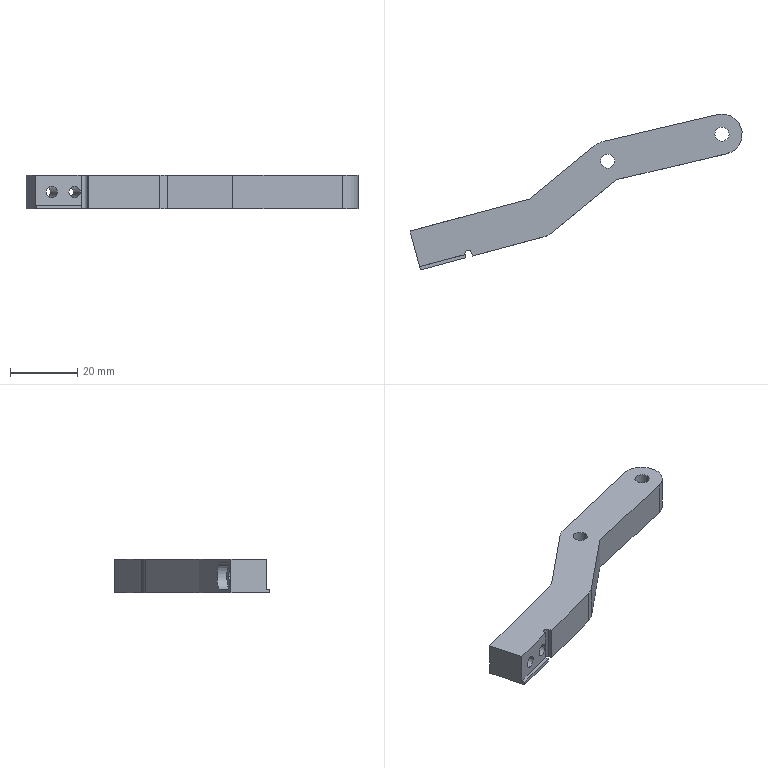Part | STEP file | 02-07 product suction plate C | 1 solid | 35 faces | box 98.778 x 46.377 x 10 mm | volume 11497 mm3 | plane 18 | cylinder 17 | commonest cylinder face diameters 3.5 x4 4.2 x4 8 x3 12 x3 10 x2 2 x1
STEP:
#1=CARTESIAN_POINT('',(-49.535,-27.425,5.));
#2=VERTEX_POINT('',#1);
#3=CARTESIAN_POINT('',(-45.672,-26.39,9.));
#4=VERTEX_POINT('',#3);
#5=CARTESIAN_POINT('',(-45.672,-26.39,5.));
#6=DIRECTION('',(-0.2588,0.9659,0.));
#7=DIRECTION('',(-0.9659,-0.2588,0.));
#8=AXIS2_PLACEMENT_3D('',#5,#6,#7);
#9=CIRCLE('',#8,4.);
#10=EDGE_CURVE('',#2,#4,#9,.T.);
#11=ORIENTED_EDGE('',*,*,#10,.F.);
#12=CARTESIAN_POINT('',(-50.312,-24.527,5.));
#13=VERTEX_POINT('',#12);
#14=CARTESIAN_POINT('',(-49.535,-27.425,5.));
#15=DIRECTION('',(-0.2588,0.9659,0.));
#16=VECTOR('',#15,1000.);
#17=LINE('',#14,#16);
#18=EDGE_CURVE('',#2,#13,#17,.T.);
#19=ORIENTED_EDGE('',*,*,#18,.T.);
#20=CARTESIAN_POINT('',(-46.448,-23.492,9.));
#21=VERTEX_POINT('',#20);
#22=CARTESIAN_POINT('',(-46.448,-23.492,5.));
#23=DIRECTION('',(-0.2588,0.9659,0.));
#24=DIRECTION('',(-0.9659,-0.2588,0.));
#25=AXIS2_PLACEMENT_3D('',#22,#23,#24);
#26=CIRCLE('',#25,4.);
#27=EDGE_CURVE('',#13,#21,#26,.T.);
#28=ORIENTED_EDGE('',*,*,#27,.T.);
#29=CARTESIAN_POINT('',(-45.672,-26.39,9.));
#30=DIRECTION('',(-0.2588,0.9659,0.));
#31=VECTOR('',#30,1000.);
#32=LINE('',#29,#31);
#33=EDGE_CURVE('',#4,#21,#32,.T.);
#34=ORIENTED_EDGE('',*,*,#33,.F.);
#35=EDGE_LOOP('',(#11,#19,#28,#34));
#36=FACE_OUTER_BOUND('',#35,.T.);
#37=CARTESIAN_POINT('',(-45.672,-26.39,5.));
#38=DIRECTION('',(-0.2588,0.9659,0.));
#39=DIRECTION('',(-0.9659,-0.2588,0.));
#40=AXIS2_PLACEMENT_3D('',#37,#38,#39);
#41=CYLINDRICAL_SURFACE('',#40,4.);
#42=ADVANCED_FACE('',(#36),#41,.F.);
#43=CARTESIAN_POINT('',(9.6,-4.,10.));
#44=VERTEX_POINT('',#43);
#45=CARTESIAN_POINT('',(5.4,-4.,10.));
#46=VERTEX_POINT('',#45);
#47=CARTESIAN_POINT('',(7.5,-4.,10.));
#48=DIRECTION('',(0.,0.,-1.));
#49=DIRECTION('',(-1.,0.,0.));
#50=AXIS2_PLACEMENT_3D('',#47,#48,#49);
#51=CIRCLE('',#50,2.1);
#52=EDGE_CURVE('',#44,#46,#51,.T.);
#53=ORIENTED_EDGE('',*,*,#52,.F.);
#54=CARTESIAN_POINT('',(9.6,-4.,0.));
#55=VERTEX_POINT('',#54);
#56=CARTESIAN_POINT('',(9.6,-4.,0.));
#57=DIRECTION('',(0.,0.,-1.));
#58=VECTOR('',#57,1000.);
#59=LINE('',#56,#58);
#60=EDGE_CURVE('',#44,#55,#59,.T.);
#61=ORIENTED_EDGE('',*,*,#60,.T.);
#62=CARTESIAN_POINT('',(5.4,-4.,0.));
#63=VERTEX_POINT('',#62);
#64=CARTESIAN_POINT('',(7.5,-4.,0.));
#65=DIRECTION('',(0.,0.,-1.));
#66=DIRECTION('',(-1.,0.,0.));
#67=AXIS2_PLACEMENT_3D('',#64,#65,#66);
#68=CIRCLE('',#67,2.1);
#69=EDGE_CURVE('',#55,#63,#68,.T.);
#70=ORIENTED_EDGE('',*,*,#69,.T.);
#71=CARTESIAN_POINT('',(5.4,-4.,0.));
#72=DIRECTION('',(0.,0.,-1.));
#73=VECTOR('',#72,1000.);
#74=LINE('',#71,#73);
#75=EDGE_CURVE('',#46,#63,#74,.T.);
#76=ORIENTED_EDGE('',*,*,#75,.F.);
#77=EDGE_LOOP('',(#53,#61,#70,#76));
#78=FACE_OUTER_BOUND('',#77,.T.);
#79=CARTESIAN_POINT('',(7.5,-4.,0.));
#80=DIRECTION('',(0.,0.,-1.));
#81=DIRECTION('',(-1.,0.,0.));
#82=AXIS2_PLACEMENT_3D('',#79,#80,#81);
#83=CYLINDRICAL_SURFACE('',#82,2.1);
#84=ADVANCED_FACE('',(#78),#83,.F.);
#85=CARTESIAN_POINT('',(43.6,4.,10.));
#86=VERTEX_POINT('',#85);
#87=CARTESIAN_POINT('',(39.4,4.,10.));
#88=VERTEX_POINT('',#87);
#89=CARTESIAN_POINT('',(41.5,4.,10.));
#90=DIRECTION('',(0.,0.,-1.));
#91=DIRECTION('',(-1.,0.,0.));
#92=AXIS2_PLACEMENT_3D('',#89,#90,#91);
#93=CIRCLE('',#92,2.1);
#94=EDGE_CURVE('',#86,#88,#93,.T.);
#95=ORIENTED_EDGE('',*,*,#94,.F.);
#96=CARTESIAN_POINT('',(43.6,4.,1.3));
#97=VERTEX_POINT('',#96);
#98=CARTESIAN_POINT('',(43.6,4.,0.));
#99=DIRECTION('',(0.,0.,-1.));
#100=VECTOR('',#99,1000.);
#101=LINE('',#98,#100);
#102=EDGE_CURVE('',#86,#97,#101,.T.);
#103=ORIENTED_EDGE('',*,*,#102,.T.);
#104=CARTESIAN_POINT('',(39.4,4.,1.3));
#105=VERTEX_POINT('',#104);
#106=CARTESIAN_POINT('',(41.5,4.,1.3));
#107=DIRECTION('',(0.,0.,-1.));
#108=DIRECTION('',(-1.,0.,0.));
#109=AXIS2_PLACEMENT_3D('',#106,#107,#108);
#110=CIRCLE('',#109,2.1);
#111=EDGE_CURVE('',#97,#105,#110,.T.);
#112=ORIENTED_EDGE('',*,*,#111,.T.);
#113=CARTESIAN_POINT('',(39.4,4.,0.));
#114=DIRECTION('',(0.,0.,-1.));
#115=VECTOR('',#114,1000.);
#116=LINE('',#113,#115);
#117=EDGE_CURVE('',#88,#105,#116,.T.);
#118=ORIENTED_EDGE('',*,*,#117,.F.);
#119=EDGE_LOOP('',(#95,#103,#112,#118));
#120=FACE_OUTER_BOUND('',#119,.T.);
#121=CARTESIAN_POINT('',(41.5,4.,0.));
#122=DIRECTION('',(0.,0.,-1.));
#123=DIRECTION('',(-1.,0.,0.));
#124=AXIS2_PLACEMENT_3D('',#121,#122,#123);
#125=CYLINDRICAL_SURFACE('',#124,2.1);
#126=ADVANCED_FACE('',(#120),#125,.F.);
#127=CARTESIAN_POINT('',(46.5,4.,1.3));
#128=VERTEX_POINT('',#127);
#129=CARTESIAN_POINT('',(36.5,4.,1.3));
#130=VERTEX_POINT('',#129);
#131=CARTESIAN_POINT('',(41.5,4.,1.3));
#132=DIRECTION('',(0.,0.,-1.));
#133=DIRECTION('',(-1.,0.,0.));
#134=AXIS2_PLACEMENT_3D('',#131,#132,#133);
#135=CIRCLE('',#134,5.);
#136=EDGE_CURVE('',#128,#130,#135,.T.);
#137=ORIENTED_EDGE('',*,*,#136,.F.);
#138=CARTESIAN_POINT('',(46.5,4.,0.));
#139=VERTEX_POINT('',#138);
#140=CARTESIAN_POINT('',(46.5,4.,1.3));
#141=DIRECTION('',(0.,0.,-1.));
#142=VECTOR('',#141,1000.);
#143=LINE('',#140,#142);
#144=EDGE_CURVE('',#128,#139,#143,.T.);
#145=ORIENTED_EDGE('',*,*,#144,.T.);
#146=CARTESIAN_POINT('',(36.5,4.,0.));
#147=VERTEX_POINT('',#146);
#148=CARTESIAN_POINT('',(41.5,4.,0.));
#149=DIRECTION('',(0.,0.,-1.));
#150=DIRECTION('',(-1.,0.,0.));
#151=AXIS2_PLACEMENT_3D('',#148,#149,#150);
#152=CIRCLE('',#151,5.);
#153=EDGE_CURVE('',#139,#147,#152,.T.);
#154=ORIENTED_EDGE('',*,*,#153,.T.);
#155=CARTESIAN_POINT('',(36.5,4.,1.3));
#156=DIRECTION('',(0.,0.,-1.));
#157=VECTOR('',#156,1000.);
#158=LINE('',#155,#157);
#159=EDGE_CURVE('',#130,#147,#158,.T.);
#160=ORIENTED_EDGE('',*,*,#159,.F.);
#161=EDGE_LOOP('',(#137,#145,#154,#160));
#162=FACE_OUTER_BOUND('',#161,.T.);
#163=CARTESIAN_POINT('',(41.5,4.,1.3));
#164=DIRECTION('',(0.,0.,-1.));
#165=DIRECTION('',(-1.,0.,0.));
#166=AXIS2_PLACEMENT_3D('',#163,#164,#165);
#167=CYLINDRICAL_SURFACE('',#166,5.);
#168=ADVANCED_FACE('',(#162),#167,.F.);
#169=CARTESIAN_POINT('',(-35.149,-31.852,5.));
#170=VERTEX_POINT('',#169);
#171=CARTESIAN_POINT('',(-38.53,-32.758,5.));
#172=VERTEX_POINT('',#171);
#173=CARTESIAN_POINT('',(-36.84,-32.305,5.));
#174=DIRECTION('',(-0.2588,0.9659,0.));
#175=DIRECTION('',(-0.9659,-0.2588,0.));
#176=AXIS2_PLACEMENT_3D('',#173,#174,#175);
#177=CIRCLE('',#176,1.75);
#178=EDGE_CURVE('',#170,#172,#177,.T.);
#179=ORIENTED_EDGE('',*,*,#178,.F.);
#180=CARTESIAN_POINT('',(-37.22,-24.125,5.));
#181=VERTEX_POINT('',#180);
#182=CARTESIAN_POINT('',(-34.89,-32.818,5.));
#183=DIRECTION('',(-0.2588,0.9659,0.));
#184=VECTOR('',#183,1000.);
#185=LINE('',#182,#184);
#186=EDGE_CURVE('',#170,#181,#185,.T.);
#187=ORIENTED_EDGE('',*,*,#186,.T.);
#188=CARTESIAN_POINT('',(-40.601,-25.031,5.));
#189=VERTEX_POINT('',#188);
#190=CARTESIAN_POINT('',(-38.91,-24.578,5.));
#191=DIRECTION('',(0.2588,-0.9659,0.));
#192=DIRECTION('',(-0.9659,-0.2588,0.));
#193=AXIS2_PLACEMENT_3D('',#190,#191,#192);
#194=CIRCLE('',#193,1.75);
#195=EDGE_CURVE('',#189,#181,#194,.T.);
#196=ORIENTED_EDGE('',*,*,#195,.F.);
#197=CARTESIAN_POINT('',(-38.271,-33.724,5.));
#198=DIRECTION('',(-0.2588,0.9659,0.));
#199=VECTOR('',#198,1000.);
#200=LINE('',#197,#199);
#201=EDGE_CURVE('',#172,#189,#200,.T.);
#202=ORIENTED_EDGE('',*,*,#201,.F.);
#203=EDGE_LOOP('',(#179,#187,#196,#202));
#204=FACE_OUTER_BOUND('',#203,.T.);
#205=CARTESIAN_POINT('',(-36.581,-33.271,5.));
#206=DIRECTION('',(-0.2588,0.9659,0.));
#207=DIRECTION('',(-0.9659,-0.2588,0.));
#208=AXIS2_PLACEMENT_3D('',#205,#206,#207);
#209=CYLINDRICAL_SURFACE('',#208,1.75);
#210=ADVANCED_FACE('',(#204),#209,.F.);
#211=CARTESIAN_POINT('',(-41.911,-33.664,5.));
#212=VERTEX_POINT('',#211);
#213=CARTESIAN_POINT('',(-45.291,-34.57,5.));
#214=VERTEX_POINT('',#213);
#215=CARTESIAN_POINT('',(-43.601,-34.117,5.));
#216=DIRECTION('',(-0.2588,0.9659,0.));
#217=DIRECTION('',(-0.9659,-0.2588,0.));
#218=AXIS2_PLACEMENT_3D('',#215,#216,#217);
#219=CIRCLE('',#218,1.75);
#220=EDGE_CURVE('',#212,#214,#219,.T.);
#221=ORIENTED_EDGE('',*,*,#220,.F.);
#222=CARTESIAN_POINT('',(-43.981,-25.937,5.));
#223=VERTEX_POINT('',#222);
#224=CARTESIAN_POINT('',(-41.652,-34.63,5.));
#225=DIRECTION('',(-0.2588,0.9659,0.));
#226=VECTOR('',#225,1000.);
#227=LINE('',#224,#226);
#228=EDGE_CURVE('',#212,#223,#227,.T.);
#229=ORIENTED_EDGE('',*,*,#228,.T.);
#230=CARTESIAN_POINT('',(-47.362,-26.842,5.));
#231=VERTEX_POINT('',#230);
#232=CARTESIAN_POINT('',(-45.672,-26.39,5.));
#233=DIRECTION('',(0.2588,-0.9659,0.));
#234=DIRECTION('',(-0.9659,-0.2588,0.));
#235=AXIS2_PLACEMENT_3D('',#232,#233,#234);
#236=CIRCLE('',#235,1.75);
#237=EDGE_CURVE('',#231,#223,#236,.T.);
#238=ORIENTED_EDGE('',*,*,#237,.F.);
#239=CARTESIAN_POINT('',(-45.033,-35.536,5.));
#240=DIRECTION('',(-0.2588,0.9659,0.));
#241=VECTOR('',#240,1000.);
#242=LINE('',#239,#241);
#243=EDGE_CURVE('',#214,#231,#242,.T.);
#244=ORIENTED_EDGE('',*,*,#243,.F.);
#245=EDGE_LOOP('',(#221,#229,#238,#244));
#246=FACE_OUTER_BOUND('',#245,.T.);
#247=CARTESIAN_POINT('',(-43.342,-35.083,5.));
#248=DIRECTION('',(-0.2588,0.9659,0.));
#249=DIRECTION('',(-0.9659,-0.2588,0.));
#250=AXIS2_PLACEMENT_3D('',#247,#248,#249);
#251=CYLINDRICAL_SURFACE('',#250,1.75);
#252=ADVANCED_FACE('',(#246),#251,.F.);
#253=ORIENTED_EDGE('',*,*,#228,.F.);
#254=CARTESIAN_POINT('',(-43.601,-34.117,5.));
#255=DIRECTION('',(-0.2588,0.9659,0.));
#256=DIRECTION('',(-0.9659,-0.2588,0.));
#257=AXIS2_PLACEMENT_3D('',#254,#255,#256);
#258=CIRCLE('',#257,1.75);
#259=EDGE_CURVE('',#214,#212,#258,.T.);
#260=ORIENTED_EDGE('',*,*,#259,.F.);
#261=ORIENTED_EDGE('',*,*,#243,.T.);
#262=CARTESIAN_POINT('',(-45.672,-26.39,5.));
#263=DIRECTION('',(0.2588,-0.9659,0.));
#264=DIRECTION('',(-0.9659,-0.2588,0.));
#265=AXIS2_PLACEMENT_3D('',#262,#263,#264);
#266=CIRCLE('',#265,1.75);
#267=EDGE_CURVE('',#223,#231,#266,.T.);
#268=ORIENTED_EDGE('',*,*,#267,.F.);
#269=EDGE_LOOP('',(#253,#260,#261,#268));
#270=FACE_OUTER_BOUND('',#269,.T.);
#271=CARTESIAN_POINT('',(-43.342,-35.083,5.));
#272=DIRECTION('',(-0.2588,0.9659,0.));
#273=DIRECTION('',(-0.9659,-0.2588,0.));
#274=AXIS2_PLACEMENT_3D('',#271,#272,#273);
#275=CYLINDRICAL_SURFACE('',#274,1.75);
#276=ADVANCED_FACE('',(#270),#275,.F.);
#277=ORIENTED_EDGE('',*,*,#186,.F.);
#278=CARTESIAN_POINT('',(-36.84,-32.305,5.));
#279=DIRECTION('',(-0.2588,0.9659,0.));
#280=DIRECTION('',(-0.9659,-0.2588,0.));
#281=AXIS2_PLACEMENT_3D('',#278,#279,#280);
#282=CIRCLE('',#281,1.75);
#283=EDGE_CURVE('',#172,#170,#282,.T.);
#284=ORIENTED_EDGE('',*,*,#283,.F.);
#285=ORIENTED_EDGE('',*,*,#201,.T.);
#286=CARTESIAN_POINT('',(-38.91,-24.578,5.));
#287=DIRECTION('',(0.2588,-0.9659,0.));
#288=DIRECTION('',(-0.9659,-0.2588,0.));
#289=AXIS2_PLACEMENT_3D('',#286,#287,#288);
#290=CIRCLE('',#289,1.75);
#291=EDGE_CURVE('',#181,#189,#290,.T.);
#292=ORIENTED_EDGE('',*,*,#291,.F.);
#293=EDGE_LOOP('',(#277,#284,#285,#292));
#294=FACE_OUTER_BOUND('',#293,.T.);
#295=CARTESIAN_POINT('',(-36.581,-33.271,5.));
#296=DIRECTION('',(-0.2588,0.9659,0.));
#297=DIRECTION('',(-0.9659,-0.2588,0.));
#298=AXIS2_PLACEMENT_3D('',#295,#296,#297);
#299=CYLINDRICAL_SURFACE('',#298,1.75);
#300=ADVANCED_FACE('',(#294),#299,.F.);
#301=CARTESIAN_POINT('',(-34.649,-32.754,0.));
#302=VERTEX_POINT('',#301);
#303=CARTESIAN_POINT('',(-34.649,-32.754,1.));
#304=VERTEX_POINT('',#303);
#305=CARTESIAN_POINT('',(-34.649,-32.754,0.));
#306=DIRECTION('',(0.,0.,1.));
#307=VECTOR('',#306,1000.);
#308=LINE('',#305,#307);
#309=EDGE_CURVE('',#302,#304,#308,.T.);
#310=ORIENTED_EDGE('',*,*,#309,.T.);
#311=CARTESIAN_POINT('',(-48.172,-36.377,1.));
#312=VERTEX_POINT('',#311);
#313=CARTESIAN_POINT('',(-32.717,-32.236,1.));
#314=DIRECTION('',(0.9659,0.2588,0.));
#315=VECTOR('',#314,1000.);
#316=LINE('',#313,#315);
#317=EDGE_CURVE('',#312,#304,#316,.T.);
#318=ORIENTED_EDGE('',*,*,#317,.F.);
#319=CARTESIAN_POINT('',(-48.172,-36.377,0.));
#320=VERTEX_POINT('',#319);
#321=CARTESIAN_POINT('',(-48.172,-36.377,10.));
#322=DIRECTION('',(0.,0.,-1.));
#323=VECTOR('',#322,1000.);
#324=LINE('',#321,#323);
#325=EDGE_CURVE('',#312,#320,#324,.T.);
#326=ORIENTED_EDGE('',*,*,#325,.T.);
#327=CARTESIAN_POINT('',(-10.223,-26.209,0.));
#328=DIRECTION('',(-0.9659,-0.2588,0.));
#329=VECTOR('',#328,1000.);
#330=LINE('',#327,#329);
#331=EDGE_CURVE('',#302,#320,#330,.T.);
#332=ORIENTED_EDGE('',*,*,#331,.F.);
#333=EDGE_LOOP('',(#310,#318,#326,#332));
#334=FACE_OUTER_BOUND('',#333,.T.);
#335=CARTESIAN_POINT('',(-10.223,-26.209,10.));
#336=DIRECTION('',(0.2588,-0.9659,0.));
#337=DIRECTION('',(0.9659,0.2588,0.));
#338=AXIS2_PLACEMENT_3D('',#335,#336,#337);
#339=PLANE('',#338);
#340=ADVANCED_FACE('',(#334),#339,.T.);
#341=CARTESIAN_POINT('',(10.221,-9.524,10.));
#342=VERTEX_POINT('',#341);
#343=CARTESIAN_POINT('',(-9.226,-25.395,10.));
#344=VERTEX_POINT('',#343);
#345=CARTESIAN_POINT('',(10.221,-9.524,10.));
#346=DIRECTION('',(-0.7747,-0.6323,0.));
#347=VECTOR('',#346,1000.);
#348=LINE('',#345,#347);
#349=EDGE_CURVE('',#342,#344,#348,.T.);
#350=ORIENTED_EDGE('',*,*,#349,.T.);
#351=CARTESIAN_POINT('',(-9.226,-25.395,0.));
#352=VERTEX_POINT('',#351);
#353=CARTESIAN_POINT('',(-9.226,-25.395,10.));
#354=DIRECTION('',(0.,0.,-1.));
#355=VECTOR('',#354,1000.);
#356=LINE('',#353,#355);
#357=EDGE_CURVE('',#344,#352,#356,.T.);
#358=ORIENTED_EDGE('',*,*,#357,.T.);
#359=CARTESIAN_POINT('',(10.221,-9.524,0.));
#360=VERTEX_POINT('',#359);
#361=CARTESIAN_POINT('',(10.221,-9.524,0.));
#362=DIRECTION('',(-0.7747,-0.6323,0.));
#363=VECTOR('',#362,1000.);
#364=LINE('',#361,#363);
#365=EDGE_CURVE('',#360,#352,#364,.T.);
#366=ORIENTED_EDGE('',*,*,#365,.F.);
#367=CARTESIAN_POINT('',(10.221,-9.524,10.));
#368=DIRECTION('',(0.,0.,-1.));
#369=VECTOR('',#368,1000.);
#370=LINE('',#367,#369);
#371=EDGE_CURVE('',#342,#360,#370,.T.);
#372=ORIENTED_EDGE('',*,*,#371,.F.);
#373=EDGE_LOOP('',(#350,#358,#366,#372));
#374=FACE_OUTER_BOUND('',#373,.T.);
#375=CARTESIAN_POINT('',(10.221,-9.524,10.));
#376=DIRECTION('',(0.6323,-0.7747,0.));
#377=DIRECTION('',(0.7747,0.6323,0.));
#378=AXIS2_PLACEMENT_3D('',#375,#376,#377);
#379=PLANE('',#378);
#380=ADVANCED_FACE('',(#374),#379,.T.);
#381=CARTESIAN_POINT('',(42.874,-1.841,0.));
#382=VERTEX_POINT('',#381);
#383=CARTESIAN_POINT('',(42.874,-1.841,0.));
#384=DIRECTION('',(-0.9734,-0.229,0.));
#385=VECTOR('',#384,1000.);
#386=LINE('',#383,#385);
#387=EDGE_CURVE('',#382,#360,#386,.T.);
#388=ORIENTED_EDGE('',*,*,#387,.F.);
#389=CARTESIAN_POINT('',(42.874,-1.841,10.));
#390=VERTEX_POINT('',#389);
#391=CARTESIAN_POINT('',(42.874,-1.841,10.));
#392=DIRECTION('',(0.,0.,-1.));
#393=VECTOR('',#392,1000.);
#394=LINE('',#391,#393);
#395=EDGE_CURVE('',#390,#382,#394,.T.);
#396=ORIENTED_EDGE('',*,*,#395,.F.);
#397=CARTESIAN_POINT('',(42.874,-1.841,10.));
#398=DIRECTION('',(-0.9734,-0.229,0.));
#399=VECTOR('',#398,1000.);
#400=LINE('',#397,#399);
#401=EDGE_CURVE('',#390,#342,#400,.T.);
#402=ORIENTED_EDGE('',*,*,#401,.T.);
#403=ORIENTED_EDGE('',*,*,#371,.T.);
#404=EDGE_LOOP('',(#388,#396,#402,#403));
#405=FACE_OUTER_BOUND('',#404,.T.);
#406=CARTESIAN_POINT('',(42.874,-1.841,10.));
#407=DIRECTION('',(0.229,-0.9734,0.));
#408=DIRECTION('',(0.9734,0.229,0.));
#409=AXIS2_PLACEMENT_3D('',#406,#407,#408);
#410=PLANE('',#409);
#411=ADVANCED_FACE('',(#405),#410,.T.);
#412=CARTESIAN_POINT('',(40.126,9.841,0.));
#413=VERTEX_POINT('',#412);
#414=CARTESIAN_POINT('',(41.5,4.,0.));
#415=DIRECTION('',(0.,0.,-1.));
#416=DIRECTION('',(-1.,0.,0.));
#417=AXIS2_PLACEMENT_3D('',#414,#415,#416);
#418=CIRCLE('',#417,6.);
#419=EDGE_CURVE('',#413,#382,#418,.T.);
#420=ORIENTED_EDGE('',*,*,#419,.F.);
#421=CARTESIAN_POINT('',(40.126,9.841,10.));
#422=VERTEX_POINT('',#421);
#423=CARTESIAN_POINT('',(40.126,9.841,10.));
#424=DIRECTION('',(0.,0.,-1.));
#425=VECTOR('',#424,1000.);
#426=LINE('',#423,#425);
#427=EDGE_CURVE('',#422,#413,#426,.T.);
#428=ORIENTED_EDGE('',*,*,#427,.F.);
#429=CARTESIAN_POINT('',(41.5,4.,10.));
#430=DIRECTION('',(0.,0.,-1.));
#431=DIRECTION('',(-1.,0.,0.));
#432=AXIS2_PLACEMENT_3D('',#429,#430,#431);
#433=CIRCLE('',#432,6.);
#434=EDGE_CURVE('',#422,#390,#433,.T.);
#435=ORIENTED_EDGE('',*,*,#434,.T.);
#436=ORIENTED_EDGE('',*,*,#395,.T.);
#437=EDGE_LOOP('',(#420,#428,#435,#436));
#438=FACE_OUTER_BOUND('',#437,.T.);
#439=CARTESIAN_POINT('',(41.5,4.,10.));
#440=DIRECTION('',(0.,0.,-1.));
#441=DIRECTION('',(-1.,0.,0.));
#442=AXIS2_PLACEMENT_3D('',#439,#440,#441);
#443=CYLINDRICAL_SURFACE('',#442,6.);
#444=ADVANCED_FACE('',(#438),#443,.T.);
#445=CARTESIAN_POINT('',(6.126,1.841,0.));
#446=VERTEX_POINT('',#445);
#447=CARTESIAN_POINT('',(-54.585,-12.444,0.));
#448=DIRECTION('',(0.9734,0.229,0.));
#449=VECTOR('',#448,1000.);
#450=LINE('',#447,#449);
#451=EDGE_CURVE('',#446,#413,#450,.T.);
#452=ORIENTED_EDGE('',*,*,#451,.F.);
#453=CARTESIAN_POINT('',(6.126,1.841,10.));
#454=VERTEX_POINT('',#453);
#455=CARTESIAN_POINT('',(6.126,1.841,10.));
#456=DIRECTION('',(0.,0.,1.));
#457=VECTOR('',#456,1000.);
#458=LINE('',#455,#457);
#459=EDGE_CURVE('',#446,#454,#458,.T.);
#460=ORIENTED_EDGE('',*,*,#459,.T.);
#461=CARTESIAN_POINT('',(-54.585,-12.444,10.));
#462=DIRECTION('',(0.9734,0.229,0.));
#463=VECTOR('',#462,1000.);
#464=LINE('',#461,#463);
#465=EDGE_CURVE('',#454,#422,#464,.T.);
#466=ORIENTED_EDGE('',*,*,#465,.T.);
#467=ORIENTED_EDGE('',*,*,#427,.T.);
#468=EDGE_LOOP('',(#452,#460,#466,#467));
#469=FACE_OUTER_BOUND('',#468,.T.);
#470=CARTESIAN_POINT('',(-54.585,-12.444,10.));
#471=DIRECTION('',(-0.229,0.9734,0.));
#472=DIRECTION('',(-0.9734,-0.229,0.));
#473=AXIS2_PLACEMENT_3D('',#470,#471,#472);
#474=PLANE('',#473);
#475=ADVANCED_FACE('',(#469),#474,.T.);
#476=CARTESIAN_POINT('',(-48.431,-35.411,1.));
#477=VERTEX_POINT('',#476);
#478=CARTESIAN_POINT('',(-48.431,-35.411,10.));
#479=VERTEX_POINT('',#478);
#480=CARTESIAN_POINT('',(-48.431,-35.411,1.));
#481=DIRECTION('',(0.,0.,1.));
#482=VECTOR('',#481,1000.);
#483=LINE('',#480,#482);
#484=EDGE_CURVE('',#477,#479,#483,.T.);
#485=ORIENTED_EDGE('',*,*,#484,.T.);
#486=CARTESIAN_POINT('',(-51.278,-24.786,10.));
#487=VERTEX_POINT('',#486);
#488=CARTESIAN_POINT('',(-48.172,-36.377,10.));
#489=DIRECTION('',(-0.2588,0.9659,0.));
#490=VECTOR('',#489,1000.);
#491=LINE('',#488,#490);
#492=EDGE_CURVE('',#479,#487,#491,.T.);
#493=ORIENTED_EDGE('',*,*,#492,.T.);
#494=CARTESIAN_POINT('',(-51.278,-24.786,0.));
#495=VERTEX_POINT('',#494);
#496=CARTESIAN_POINT('',(-51.278,-24.786,0.));
#497=DIRECTION('',(0.,0.,1.));
#498=VECTOR('',#497,1000.);
#499=LINE('',#496,#498);
#500=EDGE_CURVE('',#495,#487,#499,.T.);
#501=ORIENTED_EDGE('',*,*,#500,.F.);
#502=CARTESIAN_POINT('',(-48.172,-36.377,0.));
#503=DIRECTION('',(-0.2588,0.9659,0.));
#504=VECTOR('',#503,1000.);
#505=LINE('',#502,#504);
#506=EDGE_CURVE('',#320,#495,#505,.T.);
#507=ORIENTED_EDGE('',*,*,#506,.F.);
#508=ORIENTED_EDGE('',*,*,#325,.F.);
#509=CARTESIAN_POINT('',(-48.172,-36.377,1.));
#510=DIRECTION('',(0.2588,-0.9659,0.));
#511=VECTOR('',#510,1000.);
#512=LINE('',#509,#511);
#513=EDGE_CURVE('',#477,#312,#512,.T.);
#514=ORIENTED_EDGE('',*,*,#513,.F.);
#515=EDGE_LOOP('',(#485,#493,#501,#507,#508,#514));
#516=FACE_OUTER_BOUND('',#515,.T.);
#517=CARTESIAN_POINT('',(-48.172,-36.377,10.));
#518=DIRECTION('',(-0.9659,-0.2588,0.));
#519=DIRECTION('',(0.2588,-0.9659,0.));
#520=AXIS2_PLACEMENT_3D('',#517,#518,#519);
#521=PLANE('',#520);
#522=ADVANCED_FACE('',(#516),#521,.T.);
#523=CARTESIAN_POINT('',(-32.717,-32.236,0.));
#524=VERTEX_POINT('',#523);
#525=CARTESIAN_POINT('',(-32.717,-32.236,10.));
#526=VERTEX_POINT('',#525);
#527=CARTESIAN_POINT('',(-32.717,-32.236,1.));
#528=DIRECTION('',(0.,0.,1.));
#529=VECTOR('',#528,1000.);
#530=LINE('',#527,#529);
#531=EDGE_CURVE('',#524,#526,#530,.T.);
#532=ORIENTED_EDGE('',*,*,#531,.F.);
#533=CARTESIAN_POINT('',(-11.467,-26.542,0.));
#534=VERTEX_POINT('',#533);
#535=CARTESIAN_POINT('',(-10.223,-26.209,0.));
#536=DIRECTION('',(-0.9659,-0.2588,0.));
#537=VECTOR('',#536,1000.);
#538=LINE('',#535,#537);
#539=EDGE_CURVE('',#534,#524,#538,.T.);
#540=ORIENTED_EDGE('',*,*,#539,.F.);
#541=CARTESIAN_POINT('',(-11.467,-26.542,10.));
#542=VERTEX_POINT('',#541);
#543=CARTESIAN_POINT('',(-11.467,-26.542,10.));
#544=DIRECTION('',(0.,0.,1.));
#545=VECTOR('',#544,1000.);
#546=LINE('',#543,#545);
#547=EDGE_CURVE('',#534,#542,#546,.T.);
#548=ORIENTED_EDGE('',*,*,#547,.T.);
#549=CARTESIAN_POINT('',(-10.223,-26.209,10.));
#550=DIRECTION('',(-0.9659,-0.2588,0.));
#551=VECTOR('',#550,1000.);
#552=LINE('',#549,#551);
#553=EDGE_CURVE('',#542,#526,#552,.T.);
#554=ORIENTED_EDGE('',*,*,#553,.T.);
#555=EDGE_LOOP('',(#532,#540,#548,#554));
#556=FACE_OUTER_BOUND('',#555,.T.);
#557=CARTESIAN_POINT('',(-10.223,-26.209,10.));
#558=DIRECTION('',(0.2588,-0.9659,0.));
#559=DIRECTION('',(0.9659,0.2588,0.));
#560=AXIS2_PLACEMENT_3D('',#557,#558,#559);
#561=PLANE('',#560);
#562=ADVANCED_FACE('',(#556),#561,.T.);
#563=CARTESIAN_POINT('',(7.5,-4.,10.));
#564=DIRECTION('',(0.,0.,-1.));
#565=DIRECTION('',(-1.,0.,0.));
#566=AXIS2_PLACEMENT_3D('',#563,#564,#565);
#567=CIRCLE('',#566,2.1);
#568=EDGE_CURVE('',#46,#44,#567,.T.);
#569=ORIENTED_EDGE('',*,*,#568,.T.);
#570=ORIENTED_EDGE('',*,*,#52,.T.);
#571=EDGE_LOOP('',(#569,#570));
#572=FACE_BOUND('',#571,.T.);
#573=CARTESIAN_POINT('',(41.5,4.,10.));
#574=DIRECTION('',(0.,0.,-1.));
#575=DIRECTION('',(-1.,0.,0.));
#576=AXIS2_PLACEMENT_3D('',#573,#574,#575);
#577=CIRCLE('',#576,2.1);
#578=EDGE_CURVE('',#88,#86,#577,.T.);
#579=ORIENTED_EDGE('',*,*,#578,.T.);
#580=ORIENTED_EDGE('',*,*,#94,.T.);
#581=EDGE_LOOP('',(#579,#580));
#582=FACE_BOUND('',#581,.T.);
#583=CARTESIAN_POINT('',(-34.908,-31.788,10.));
#584=VERTEX_POINT('',#583);
#585=CARTESIAN_POINT('',(-48.431,-35.411,10.));
#586=DIRECTION('',(-0.9659,-0.2588,0.));
#587=VECTOR('',#586,1000.);
#588=LINE('',#585,#587);
#589=EDGE_CURVE('',#584,#479,#588,.T.);
#590=ORIENTED_EDGE('',*,*,#589,.F.);
#591=CARTESIAN_POINT('',(-32.976,-31.27,10.));
#592=VERTEX_POINT('',#591);
#593=CARTESIAN_POINT('',(-33.942,-31.529,10.));
#594=DIRECTION('',(0.,0.,1.));
#595=DIRECTION('',(1.,0.,0.));
#596=AXIS2_PLACEMENT_3D('',#593,#594,#595);
#597=CIRCLE('',#596,1.);
#598=EDGE_CURVE('',#592,#584,#597,.T.);
#599=ORIENTED_EDGE('',*,*,#598,.F.);
#600=CARTESIAN_POINT('',(-32.976,-31.27,10.));
#601=DIRECTION('',(-0.2588,0.9659,0.));
#602=VECTOR('',#601,1000.);
#603=LINE('',#600,#602);
#604=EDGE_CURVE('',#526,#592,#603,.T.);
#605=ORIENTED_EDGE('',*,*,#604,.F.);
#606=ORIENTED_EDGE('',*,*,#553,.F.);
#607=CARTESIAN_POINT('',(-13.02,-20.746,10.));
#608=DIRECTION('',(0.,0.,1.));
#609=DIRECTION('',(-1.,0.,0.));
#610=AXIS2_PLACEMENT_3D('',#607,#608,#609);
#611=CIRCLE('',#610,6.);
#612=EDGE_CURVE('',#542,#344,#611,.T.);
#613=ORIENTED_EDGE('',*,*,#612,.T.);
#614=ORIENTED_EDGE('',*,*,#349,.F.);
#615=ORIENTED_EDGE('',*,*,#401,.F.);
#616=ORIENTED_EDGE('',*,*,#434,.F.);
#617=ORIENTED_EDGE('',*,*,#465,.F.);
#618=CARTESIAN_POINT('',(3.706,0.6485,10.));
#619=VERTEX_POINT('',#618);
#620=CARTESIAN_POINT('',(7.5,-4.,10.));
#621=DIRECTION('',(0.,0.,1.));
#622=DIRECTION('',(-1.,0.,0.));
#623=AXIS2_PLACEMENT_3D('',#620,#621,#622);
#624=CIRCLE('',#623,6.);
#625=EDGE_CURVE('',#454,#619,#624,.T.);
#626=ORIENTED_EDGE('',*,*,#625,.T.);
#627=CARTESIAN_POINT('',(-15.816,-15.284,10.));
#628=VERTEX_POINT('',#627);
#629=CARTESIAN_POINT('',(-15.816,-15.284,10.));
#630=DIRECTION('',(0.7747,0.6323,0.));
#631=VECTOR('',#630,1000.);
#632=LINE('',#629,#631);
#633=EDGE_CURVE('',#628,#619,#632,.T.);
#634=ORIENTED_EDGE('',*,*,#633,.F.);
#635=CARTESIAN_POINT('',(-51.278,-24.786,10.));
#636=DIRECTION('',(0.9659,0.2588,0.));
#637=VECTOR('',#636,1000.);
#638=LINE('',#635,#637);
#639=EDGE_CURVE('',#487,#628,#638,.T.);
#640=ORIENTED_EDGE('',*,*,#639,.F.);
#641=ORIENTED_EDGE('',*,*,#492,.F.);
#642=EDGE_LOOP('',(#590,#599,#605,#606,#613,#614,#615,#616,#617,#626,#634,#640,#641));
#643=FACE_OUTER_BOUND('',#642,.T.);
#644=CARTESIAN_POINT('',(41.5,4.,10.));
#645=DIRECTION('',(0.,0.,-1.));
#646=DIRECTION('',(-1.,0.,0.));
#647=AXIS2_PLACEMENT_3D('',#644,#645,#646);
#648=PLANE('',#647);
#649=ADVANCED_FACE('',(#572,#582,#643),#648,.F.);
#650=CARTESIAN_POINT('',(-34.908,-31.788,0.));
#651=VERTEX_POINT('',#650);
#652=CARTESIAN_POINT('',(-34.908,-31.788,0.));
#653=DIRECTION('',(0.2588,-0.9659,0.));
#654=VECTOR('',#653,1000.);
#655=LINE('',#652,#654);
#656=EDGE_CURVE('',#651,#302,#655,.T.);
#657=ORIENTED_EDGE('',*,*,#656,.T.);
#658=ORIENTED_EDGE('',*,*,#331,.T.);
#659=ORIENTED_EDGE('',*,*,#506,.T.);
#660=CARTESIAN_POINT('',(-15.816,-15.284,0.));
#661=VERTEX_POINT('',#660);
#662=CARTESIAN_POINT('',(-51.278,-24.786,0.));
#663=DIRECTION('',(0.9659,0.2588,0.));
#664=VECTOR('',#663,1000.);
#665=LINE('',#662,#664);
#666=EDGE_CURVE('',#495,#661,#665,.T.);
#667=ORIENTED_EDGE('',*,*,#666,.T.);
#668=CARTESIAN_POINT('',(3.706,0.6485,0.));
#669=VERTEX_POINT('',#668);
#670=CARTESIAN_POINT('',(-15.816,-15.284,0.));
#671=DIRECTION('',(0.7747,0.6323,0.));
#672=VECTOR('',#671,1000.);
#673=LINE('',#670,#672);
#674=EDGE_CURVE('',#661,#669,#673,.T.);
#675=ORIENTED_EDGE('',*,*,#674,.T.);
#676=CARTESIAN_POINT('',(7.5,-4.,0.));
#677=DIRECTION('',(0.,0.,-1.));
#678=DIRECTION('',(-1.,0.,0.));
#679=AXIS2_PLACEMENT_3D('',#676,#677,#678);
#680=CIRCLE('',#679,6.);
#681=EDGE_CURVE('',#669,#446,#680,.T.);
#682=ORIENTED_EDGE('',*,*,#681,.T.);
#683=ORIENTED_EDGE('',*,*,#451,.T.);
#684=ORIENTED_EDGE('',*,*,#419,.T.);
#685=ORIENTED_EDGE('',*,*,#387,.T.);
#686=ORIENTED_EDGE('',*,*,#365,.T.);
#687=CARTESIAN_POINT('',(-13.02,-20.746,0.));
#688=DIRECTION('',(0.,0.,-1.));
#689=DIRECTION('',(-1.,0.,0.));
#690=AXIS2_PLACEMENT_3D('',#687,#688,#689);
#691=CIRCLE('',#690,6.);
#692=EDGE_CURVE('',#352,#534,#691,.T.);
#693=ORIENTED_EDGE('',*,*,#692,.T.);
#694=ORIENTED_EDGE('',*,*,#539,.T.);
#695=CARTESIAN_POINT('',(-32.976,-31.27,0.));
#696=VERTEX_POINT('',#695);
#697=CARTESIAN_POINT('',(-32.717,-32.236,0.));
#698=DIRECTION('',(-0.2588,0.9659,0.));
#699=VECTOR('',#698,1000.);
#700=LINE('',#697,#699);
#701=EDGE_CURVE('',#524,#696,#700,.T.);
#702=ORIENTED_EDGE('',*,*,#701,.T.);
#703=CARTESIAN_POINT('',(-33.942,-31.529,0.));
#704=DIRECTION('',(0.,0.,1.));
#705=DIRECTION('',(1.,0.,0.));
#706=AXIS2_PLACEMENT_3D('',#703,#704,#705);
#707=CIRCLE('',#706,1.);
#708=EDGE_CURVE('',#696,#651,#707,.T.);
#709=ORIENTED_EDGE('',*,*,#708,.T.);
#710=EDGE_LOOP('',(#657,#658,#659,#667,#675,#682,#683,#684,#685,#686,#693,#694,#702,#709));
#711=FACE_OUTER_BOUND('',#710,.T.);
#712=CARTESIAN_POINT('',(7.5,-4.,0.));
#713=DIRECTION('',(0.,0.,-1.));
#714=DIRECTION('',(-1.,0.,0.));
#715=AXIS2_PLACEMENT_3D('',#712,#713,#714);
#716=CIRCLE('',#715,2.1);
#717=EDGE_CURVE('',#63,#55,#716,.T.);
#718=ORIENTED_EDGE('',*,*,#717,.F.);
#719=ORIENTED_EDGE('',*,*,#69,.F.);
#720=EDGE_LOOP('',(#718,#719));
#721=FACE_BOUND('',#720,.T.);
#722=CARTESIAN_POINT('',(41.5,4.,0.));
#723=DIRECTION('',(0.,0.,-1.));
#724=DIRECTION('',(-1.,0.,0.));
#725=AXIS2_PLACEMENT_3D('',#722,#723,#724);
#726=CIRCLE('',#725,5.);
#727=EDGE_CURVE('',#147,#139,#726,.T.);
#728=ORIENTED_EDGE('',*,*,#727,.F.);
#729=ORIENTED_EDGE('',*,*,#153,.F.);
#730=EDGE_LOOP('',(#728,#729));
#731=FACE_BOUND('',#730,.T.);
#732=CARTESIAN_POINT('',(41.5,4.,0.));
#733=DIRECTION('',(0.,0.,-1.));
#734=DIRECTION('',(-1.,0.,0.));
#735=AXIS2_PLACEMENT_3D('',#732,#733,#734);
#736=PLANE('',#735);
#737=ADVANCED_FACE('',(#711,#721,#731),#736,.T.);
#738=CARTESIAN_POINT('',(-39.687,-21.68,9.));
#739=VERTEX_POINT('',#738);
#740=CARTESIAN_POINT('',(-46.448,-23.492,9.));
#741=DIRECTION('',(0.9659,0.2588,0.));
#742=VECTOR('',#741,1000.);
#743=LINE('',#740,#742);
#744=EDGE_CURVE('',#21,#739,#743,.T.);
#745=ORIENTED_EDGE('',*,*,#744,.F.);
#746=ORIENTED_EDGE('',*,*,#27,.F.);
#747=CARTESIAN_POINT('',(-46.448,-23.492,1.));
#748=VERTEX_POINT('',#747);
#749=CARTESIAN_POINT('',(-46.448,-23.492,5.));
#750=DIRECTION('',(-0.2588,0.9659,0.));
#751=DIRECTION('',(-0.9659,-0.2588,0.));
#752=AXIS2_PLACEMENT_3D('',#749,#750,#751);
#753=CIRCLE('',#752,4.);
#754=EDGE_CURVE('',#748,#13,#753,.T.);
#755=ORIENTED_EDGE('',*,*,#754,.F.);
#756=CARTESIAN_POINT('',(-39.687,-21.68,1.));
#757=VERTEX_POINT('',#756);
#758=CARTESIAN_POINT('',(-46.448,-23.492,1.));
#759=DIRECTION('',(-0.9659,-0.2588,0.));
#760=VECTOR('',#759,1000.);
#761=LINE('',#758,#760);
#762=EDGE_CURVE('',#757,#748,#761,.T.);
#763=ORIENTED_EDGE('',*,*,#762,.F.);
#764=CARTESIAN_POINT('',(-39.687,-21.68,5.));
#765=DIRECTION('',(-0.2588,0.9659,0.));
#766=DIRECTION('',(-0.9659,-0.2588,0.));
#767=AXIS2_PLACEMENT_3D('',#764,#765,#766);
#768=CIRCLE('',#767,4.);
#769=EDGE_CURVE('',#739,#757,#768,.T.);
#770=ORIENTED_EDGE('',*,*,#769,.F.);
#771=EDGE_LOOP('',(#745,#746,#755,#763,#770));
#772=FACE_BOUND('',#771,.T.);
#773=ORIENTED_EDGE('',*,*,#639,.T.);
#774=CARTESIAN_POINT('',(-15.816,-15.284,0.));
#775=DIRECTION('',(0.,0.,1.));
#776=VECTOR('',#775,1000.);
#777=LINE('',#774,#776);
#778=EDGE_CURVE('',#661,#628,#777,.T.);
#779=ORIENTED_EDGE('',*,*,#778,.F.);
#780=ORIENTED_EDGE('',*,*,#666,.F.);
#781=ORIENTED_EDGE('',*,*,#500,.T.);
#782=EDGE_LOOP('',(#773,#779,#780,#781));
#783=FACE_OUTER_BOUND('',#782,.T.);
#784=CARTESIAN_POINT('',(-51.278,-24.786,0.));
#785=DIRECTION('',(0.2588,-0.9659,0.));
#786=DIRECTION('',(0.9659,0.2588,0.));
#787=AXIS2_PLACEMENT_3D('',#784,#785,#786);
#788=PLANE('',#787);
#789=ADVANCED_FACE('',(#772,#783),#788,.F.);
#790=ORIENTED_EDGE('',*,*,#633,.T.);
#791=CARTESIAN_POINT('',(3.706,0.6485,0.));
#792=DIRECTION('',(0.,0.,-1.));
#793=VECTOR('',#792,1000.);
#794=LINE('',#791,#793);
#795=EDGE_CURVE('',#619,#669,#794,.T.);
#796=ORIENTED_EDGE('',*,*,#795,.T.);
#797=ORIENTED_EDGE('',*,*,#674,.F.);
#798=ORIENTED_EDGE('',*,*,#778,.T.);
#799=EDGE_LOOP('',(#790,#796,#797,#798));
#800=FACE_OUTER_BOUND('',#799,.T.);
#801=CARTESIAN_POINT('',(-15.816,-15.284,0.));
#802=DIRECTION('',(0.6323,-0.7747,0.));
#803=DIRECTION('',(0.7747,0.6323,0.));
#804=AXIS2_PLACEMENT_3D('',#801,#802,#803);
#805=PLANE('',#804);
#806=ADVANCED_FACE('',(#800),#805,.F.);
#807=ORIENTED_EDGE('',*,*,#144,.F.);
#808=CARTESIAN_POINT('',(41.5,4.,1.3));
#809=DIRECTION('',(0.,0.,-1.));
#810=DIRECTION('',(-1.,0.,0.));
#811=AXIS2_PLACEMENT_3D('',#808,#809,#810);
#812=CIRCLE('',#811,5.);
#813=EDGE_CURVE('',#130,#128,#812,.T.);
#814=ORIENTED_EDGE('',*,*,#813,.F.);
#815=ORIENTED_EDGE('',*,*,#159,.T.);
#816=ORIENTED_EDGE('',*,*,#727,.T.);
#817=EDGE_LOOP('',(#807,#814,#815,#816));
#818=FACE_OUTER_BOUND('',#817,.T.);
#819=CARTESIAN_POINT('',(41.5,4.,1.3));
#820=DIRECTION('',(0.,0.,-1.));
#821=DIRECTION('',(-1.,0.,0.));
#822=AXIS2_PLACEMENT_3D('',#819,#820,#821);
#823=CYLINDRICAL_SURFACE('',#822,5.);
#824=ADVANCED_FACE('',(#818),#823,.F.);
#825=CARTESIAN_POINT('',(41.5,4.,1.3));
#826=DIRECTION('',(0.,0.,-1.));
#827=DIRECTION('',(-1.,0.,0.));
#828=AXIS2_PLACEMENT_3D('',#825,#826,#827);
#829=CIRCLE('',#828,2.1);
#830=EDGE_CURVE('',#105,#97,#829,.T.);
#831=ORIENTED_EDGE('',*,*,#830,.F.);
#832=ORIENTED_EDGE('',*,*,#111,.F.);
#833=EDGE_LOOP('',(#831,#832));
#834=FACE_BOUND('',#833,.T.);
#835=ORIENTED_EDGE('',*,*,#813,.T.);
#836=ORIENTED_EDGE('',*,*,#136,.T.);
#837=EDGE_LOOP('',(#835,#836));
#838=FACE_OUTER_BOUND('',#837,.T.);
#839=CARTESIAN_POINT('',(41.5,4.,1.3));
#840=DIRECTION('',(0.,0.,-1.));
#841=DIRECTION('',(-1.,0.,0.));
#842=AXIS2_PLACEMENT_3D('',#839,#840,#841);
#843=PLANE('',#842);
#844=ADVANCED_FACE('',(#834,#838),#843,.T.);
#845=ORIENTED_EDGE('',*,*,#102,.F.);
#846=ORIENTED_EDGE('',*,*,#578,.F.);
#847=ORIENTED_EDGE('',*,*,#117,.T.);
#848=ORIENTED_EDGE('',*,*,#830,.T.);
#849=EDGE_LOOP('',(#845,#846,#847,#848));
#850=FACE_OUTER_BOUND('',#849,.T.);
#851=CARTESIAN_POINT('',(41.5,4.,0.));
#852=DIRECTION('',(0.,0.,-1.));
#853=DIRECTION('',(-1.,0.,0.));
#854=AXIS2_PLACEMENT_3D('',#851,#852,#853);
#855=CYLINDRICAL_SURFACE('',#854,2.1);
#856=ADVANCED_FACE('',(#850),#855,.F.);
#857=ORIENTED_EDGE('',*,*,#60,.F.);
#858=ORIENTED_EDGE('',*,*,#568,.F.);
#859=ORIENTED_EDGE('',*,*,#75,.T.);
#860=ORIENTED_EDGE('',*,*,#717,.T.);
#861=EDGE_LOOP('',(#857,#858,#859,#860));
#862=FACE_OUTER_BOUND('',#861,.T.);
#863=CARTESIAN_POINT('',(7.5,-4.,0.));
#864=DIRECTION('',(0.,0.,-1.));
#865=DIRECTION('',(-1.,0.,0.));
#866=AXIS2_PLACEMENT_3D('',#863,#864,#865);
#867=CYLINDRICAL_SURFACE('',#866,2.1);
#868=ADVANCED_FACE('',(#862),#867,.F.);
#869=ORIENTED_EDGE('',*,*,#681,.F.);
#870=ORIENTED_EDGE('',*,*,#795,.F.);
#871=ORIENTED_EDGE('',*,*,#625,.F.);
#872=ORIENTED_EDGE('',*,*,#459,.F.);
#873=EDGE_LOOP('',(#869,#870,#871,#872));
#874=FACE_OUTER_BOUND('',#873,.T.);
#875=CARTESIAN_POINT('',(7.5,-4.,10.));
#876=DIRECTION('',(0.,0.,-1.));
#877=DIRECTION('',(-1.,0.,0.));
#878=AXIS2_PLACEMENT_3D('',#875,#876,#877);
#879=CYLINDRICAL_SURFACE('',#878,6.);
#880=ADVANCED_FACE('',(#874),#879,.T.);
#881=ORIENTED_EDGE('',*,*,#612,.F.);
#882=ORIENTED_EDGE('',*,*,#547,.F.);
#883=ORIENTED_EDGE('',*,*,#692,.F.);
#884=ORIENTED_EDGE('',*,*,#357,.F.);
#885=EDGE_LOOP('',(#881,#882,#883,#884));
#886=FACE_OUTER_BOUND('',#885,.T.);
#887=CARTESIAN_POINT('',(-13.02,-20.746,10.));
#888=DIRECTION('',(0.,0.,-1.));
#889=DIRECTION('',(-1.,0.,0.));
#890=AXIS2_PLACEMENT_3D('',#887,#888,#889);
#891=CYLINDRICAL_SURFACE('',#890,6.);
#892=ADVANCED_FACE('',(#886),#891,.T.);
#893=ORIENTED_EDGE('',*,*,#283,.T.);
#894=ORIENTED_EDGE('',*,*,#178,.T.);
#895=EDGE_LOOP('',(#893,#894));
#896=FACE_BOUND('',#895,.T.);
#897=ORIENTED_EDGE('',*,*,#259,.T.);
#898=ORIENTED_EDGE('',*,*,#220,.T.);
#899=EDGE_LOOP('',(#897,#898));
#900=FACE_BOUND('',#899,.T.);
#901=CARTESIAN_POINT('',(-34.908,-31.788,1.));
#902=VERTEX_POINT('',#901);
#903=CARTESIAN_POINT('',(-48.431,-35.411,1.));
#904=DIRECTION('',(-0.9659,-0.2588,0.));
#905=VECTOR('',#904,1000.);
#906=LINE('',#903,#905);
#907=EDGE_CURVE('',#902,#477,#906,.T.);
#908=ORIENTED_EDGE('',*,*,#907,.F.);
#909=CARTESIAN_POINT('',(-34.908,-31.788,0.));
#910=DIRECTION('',(0.,0.,1.));
#911=VECTOR('',#910,1000.);
#912=LINE('',#909,#911);
#913=EDGE_CURVE('',#902,#584,#912,.T.);
#914=ORIENTED_EDGE('',*,*,#913,.T.);
#915=ORIENTED_EDGE('',*,*,#589,.T.);
#916=ORIENTED_EDGE('',*,*,#484,.F.);
#917=EDGE_LOOP('',(#908,#914,#915,#916));
#918=FACE_OUTER_BOUND('',#917,.T.);
#919=CARTESIAN_POINT('',(-48.431,-35.411,1.));
#920=DIRECTION('',(-0.2588,0.9659,0.));
#921=DIRECTION('',(-0.9659,-0.2588,0.));
#922=AXIS2_PLACEMENT_3D('',#919,#920,#921);
#923=PLANE('',#922);
#924=ADVANCED_FACE('',(#896,#900,#918),#923,.F.);
#925=ORIENTED_EDGE('',*,*,#604,.T.);
#926=CARTESIAN_POINT('',(-32.976,-31.27,1.));
#927=DIRECTION('',(0.,0.,1.));
#928=VECTOR('',#927,1000.);
#929=LINE('',#926,#928);
#930=EDGE_CURVE('',#696,#592,#929,.T.);
#931=ORIENTED_EDGE('',*,*,#930,.F.);
#932=ORIENTED_EDGE('',*,*,#701,.F.);
#933=ORIENTED_EDGE('',*,*,#531,.T.);
#934=EDGE_LOOP('',(#925,#931,#932,#933));
#935=FACE_OUTER_BOUND('',#934,.T.);
#936=CARTESIAN_POINT('',(-32.976,-31.27,1.));
#937=DIRECTION('',(0.9659,0.2588,0.));
#938=DIRECTION('',(-0.2588,0.9659,0.));
#939=AXIS2_PLACEMENT_3D('',#936,#937,#938);
#940=PLANE('',#939);
#941=ADVANCED_FACE('',(#935),#940,.F.);
#942=ORIENTED_EDGE('',*,*,#317,.T.);
#943=CARTESIAN_POINT('',(-34.649,-32.754,1.));
#944=DIRECTION('',(-0.2588,0.9659,0.));
#945=VECTOR('',#944,1000.);
#946=LINE('',#943,#945);
#947=EDGE_CURVE('',#304,#902,#946,.T.);
#948=ORIENTED_EDGE('',*,*,#947,.T.);
#949=ORIENTED_EDGE('',*,*,#907,.T.);
#950=ORIENTED_EDGE('',*,*,#513,.T.);
#951=EDGE_LOOP('',(#942,#948,#949,#950));
#952=FACE_OUTER_BOUND('',#951,.T.);
#953=CARTESIAN_POINT('',(-48.172,-36.377,1.));
#954=DIRECTION('',(0.,0.,-1.));
#955=DIRECTION('',(-1.,0.,0.));
#956=AXIS2_PLACEMENT_3D('',#953,#954,#955);
#957=PLANE('',#956);
#958=ADVANCED_FACE('',(#952),#957,.F.);
#959=ORIENTED_EDGE('',*,*,#309,.F.);
#960=ORIENTED_EDGE('',*,*,#656,.F.);
#961=CARTESIAN_POINT('',(-34.908,-31.788,0.));
#962=DIRECTION('',(0.,0.,1.));
#963=VECTOR('',#962,1000.);
#964=LINE('',#961,#963);
#965=EDGE_CURVE('',#651,#902,#964,.T.);
#966=ORIENTED_EDGE('',*,*,#965,.T.);
#967=ORIENTED_EDGE('',*,*,#947,.F.);
#968=EDGE_LOOP('',(#959,#960,#966,#967));
#969=FACE_OUTER_BOUND('',#968,.T.);
#970=CARTESIAN_POINT('',(-34.908,-31.788,0.));
#971=DIRECTION('',(-0.9659,-0.2588,0.));
#972=DIRECTION('',(0.2588,-0.9659,0.));
#973=AXIS2_PLACEMENT_3D('',#970,#971,#972);
#974=PLANE('',#973);
#975=ADVANCED_FACE('',(#969),#974,.F.);
#976=ORIENTED_EDGE('',*,*,#598,.T.);
#977=ORIENTED_EDGE('',*,*,#913,.F.);
#978=ORIENTED_EDGE('',*,*,#965,.F.);
#979=ORIENTED_EDGE('',*,*,#708,.F.);
#980=ORIENTED_EDGE('',*,*,#930,.T.);
#981=EDGE_LOOP('',(#976,#977,#978,#979,#980));
#982=FACE_OUTER_BOUND('',#981,.T.);
#983=CARTESIAN_POINT('',(-33.942,-31.529,0.));
#984=DIRECTION('',(0.,0.,1.));
#985=DIRECTION('',(1.,0.,0.));
#986=AXIS2_PLACEMENT_3D('',#983,#984,#985);
#987=CYLINDRICAL_SURFACE('',#986,1.);
#988=ADVANCED_FACE('',(#982),#987,.F.);
#989=ORIENTED_EDGE('',*,*,#195,.T.);
#990=ORIENTED_EDGE('',*,*,#291,.T.);
#991=EDGE_LOOP('',(#989,#990));
#992=FACE_BOUND('',#991,.T.);
#993=CARTESIAN_POINT('',(-45.672,-26.39,1.));
#994=VERTEX_POINT('',#993);
#995=CARTESIAN_POINT('',(-45.672,-26.39,5.));
#996=DIRECTION('',(-0.2588,0.9659,0.));
#997=DIRECTION('',(-0.9659,-0.2588,0.));
#998=AXIS2_PLACEMENT_3D('',#995,#996,#997);
#999=CIRCLE('',#998,4.);
#1000=EDGE_CURVE('',#994,#2,#999,.T.);
#1001=ORIENTED_EDGE('',*,*,#1000,.T.);
#1002=ORIENTED_EDGE('',*,*,#10,.T.);
#1003=CARTESIAN_POINT('',(-38.91,-24.578,9.));
#1004=VERTEX_POINT('',#1003);
#1005=CARTESIAN_POINT('',(-45.672,-26.39,9.));
#1006=DIRECTION('',(0.9659,0.2588,0.));
#1007=VECTOR('',#1006,1000.);
#1008=LINE('',#1005,#1007);
#1009=EDGE_CURVE('',#4,#1004,#1008,.T.);
#1010=ORIENTED_EDGE('',*,*,#1009,.T.);
#1011=CARTESIAN_POINT('',(-38.91,-24.578,1.));
#1012=VERTEX_POINT('',#1011);
#1013=CARTESIAN_POINT('',(-38.91,-24.578,5.));
#1014=DIRECTION('',(-0.2588,0.9659,0.));
#1015=DIRECTION('',(-0.9659,-0.2588,0.));
#1016=AXIS2_PLACEMENT_3D('',#1013,#1014,#1015);
#1017=CIRCLE('',#1016,4.);
#1018=EDGE_CURVE('',#1004,#1012,#1017,.T.);
#1019=ORIENTED_EDGE('',*,*,#1018,.T.);
#1020=CARTESIAN_POINT('',(-45.672,-26.39,1.));
#1021=DIRECTION('',(-0.9659,-0.2588,0.));
#1022=VECTOR('',#1021,1000.);
#1023=LINE('',#1020,#1022);
#1024=EDGE_CURVE('',#1012,#994,#1023,.T.);
#1025=ORIENTED_EDGE('',*,*,#1024,.T.);
#1026=EDGE_LOOP('',(#1001,#1002,#1010,#1019,#1025));
#1027=FACE_OUTER_BOUND('',#1026,.T.);
#1028=ORIENTED_EDGE('',*,*,#237,.T.);
#1029=ORIENTED_EDGE('',*,*,#267,.T.);
#1030=EDGE_LOOP('',(#1028,#1029));
#1031=FACE_BOUND('',#1030,.T.);
#1032=CARTESIAN_POINT('',(-45.672,-26.39,5.));
#1033=DIRECTION('',(-0.2588,0.9659,0.));
#1034=DIRECTION('',(-0.9659,-0.2588,0.));
#1035=AXIS2_PLACEMENT_3D('',#1032,#1033,#1034);
#1036=PLANE('',#1035);
#1037=ADVANCED_FACE('',(#992,#1027,#1031),#1036,.T.);
#1038=ORIENTED_EDGE('',*,*,#18,.F.);
#1039=ORIENTED_EDGE('',*,*,#1000,.F.);
#1040=CARTESIAN_POINT('',(-45.672,-26.39,1.));
#1041=DIRECTION('',(-0.2588,0.9659,0.));
#1042=VECTOR('',#1041,1000.);
#1043=LINE('',#1040,#1042);
#1044=EDGE_CURVE('',#994,#748,#1043,.T.);
#1045=ORIENTED_EDGE('',*,*,#1044,.T.);
#1046=ORIENTED_EDGE('',*,*,#754,.T.);
#1047=EDGE_LOOP('',(#1038,#1039,#1045,#1046));
#1048=FACE_OUTER_BOUND('',#1047,.T.);
#1049=CARTESIAN_POINT('',(-45.672,-26.39,5.));
#1050=DIRECTION('',(-0.2588,0.9659,0.));
#1051=DIRECTION('',(-0.9659,-0.2588,0.));
#1052=AXIS2_PLACEMENT_3D('',#1049,#1050,#1051);
#1053=CYLINDRICAL_SURFACE('',#1052,4.);
#1054=ADVANCED_FACE('',(#1048),#1053,.F.);
#1055=ORIENTED_EDGE('',*,*,#762,.T.);
#1056=ORIENTED_EDGE('',*,*,#1044,.F.);
#1057=ORIENTED_EDGE('',*,*,#1024,.F.);
#1058=CARTESIAN_POINT('',(-38.91,-24.578,1.));
#1059=DIRECTION('',(-0.2588,0.9659,0.));
#1060=VECTOR('',#1059,1000.);
#1061=LINE('',#1058,#1060);
#1062=EDGE_CURVE('',#1012,#757,#1061,.T.);
#1063=ORIENTED_EDGE('',*,*,#1062,.T.);
#1064=EDGE_LOOP('',(#1055,#1056,#1057,#1063));
#1065=FACE_OUTER_BOUND('',#1064,.T.);
#1066=CARTESIAN_POINT('',(-45.672,-26.39,1.));
#1067=DIRECTION('',(0.,0.,-1.));
#1068=DIRECTION('',(-1.,0.,0.));
#1069=AXIS2_PLACEMENT_3D('',#1066,#1067,#1068);
#1070=PLANE('',#1069);
#1071=ADVANCED_FACE('',(#1065),#1070,.F.);
#1072=ORIENTED_EDGE('',*,*,#769,.T.);
#1073=ORIENTED_EDGE('',*,*,#1062,.F.);
#1074=ORIENTED_EDGE('',*,*,#1018,.F.);
#1075=CARTESIAN_POINT('',(-38.91,-24.578,9.));
#1076=DIRECTION('',(-0.2588,0.9659,0.));
#1077=VECTOR('',#1076,1000.);
#1078=LINE('',#1075,#1077);
#1079=EDGE_CURVE('',#1004,#739,#1078,.T.);
#1080=ORIENTED_EDGE('',*,*,#1079,.T.);
#1081=EDGE_LOOP('',(#1072,#1073,#1074,#1080));
#1082=FACE_OUTER_BOUND('',#1081,.T.);
#1083=CARTESIAN_POINT('',(-38.91,-24.578,5.));
#1084=DIRECTION('',(-0.2588,0.9659,0.));
#1085=DIRECTION('',(-0.9659,-0.2588,0.));
#1086=AXIS2_PLACEMENT_3D('',#1083,#1084,#1085);
#1087=CYLINDRICAL_SURFACE('',#1086,4.);
#1088=ADVANCED_FACE('',(#1082),#1087,.F.);
#1089=ORIENTED_EDGE('',*,*,#744,.T.);
#1090=ORIENTED_EDGE('',*,*,#1079,.F.);
#1091=ORIENTED_EDGE('',*,*,#1009,.F.);
#1092=ORIENTED_EDGE('',*,*,#33,.T.);
#1093=EDGE_LOOP('',(#1089,#1090,#1091,#1092));
#1094=FACE_OUTER_BOUND('',#1093,.T.);
#1095=CARTESIAN_POINT('',(-45.672,-26.39,9.));
#1096=DIRECTION('',(0.,0.,1.));
#1097=DIRECTION('',(1.,0.,0.));
#1098=AXIS2_PLACEMENT_3D('',#1095,#1096,#1097);
#1099=PLANE('',#1098);
#1100=ADVANCED_FACE('',(#1094),#1099,.F.);
#1101=CLOSED_SHELL('',(#42,#84,#126,#168,#210,#252,#276,#300,#340,#380,#411,#444,#475,#522,#562,#649,#737,#789,#806,#824,#844,#856,#868,#880,#892,#924,#941,#958,#975,#988,#1037,#1054,#1071,#1088,#1100));
#1102=MANIFOLD_SOLID_BREP('',#1101);
#1103=CARTESIAN_POINT('',(0.,0.,0.));
#1104=DIRECTION('',(0.,0.,1.));
#1105=DIRECTION('',(1.,0.,0.));
#1106=AXIS2_PLACEMENT_3D('',#1103,#1104,#1105);
#1107=(LENGTH_UNIT()NAMED_UNIT(*)SI_UNIT(.MILLI.,.METRE.));
#1108=UNCERTAINTY_MEASURE_WITH_UNIT(LENGTH_MEASURE(0.00001),#1107,'','');
#1109=(NAMED_UNIT(*)PLANE_ANGLE_UNIT()SI_UNIT($,.RADIAN.));
#1110=(NAMED_UNIT(*)SI_UNIT($,.STERADIAN.)SOLID_ANGLE_UNIT());
#1111=(GEOMETRIC_REPRESENTATION_CONTEXT(3)GLOBAL_UNCERTAINTY_ASSIGNED_CONTEXT((#1108))GLOBAL_UNIT_ASSIGNED_CONTEXT((#1107,#1109,#1110))REPRESENTATION_CONTEXT('',''));
#1112=ADVANCED_BREP_SHAPE_REPRESENTATION('',(#1102,#1106),#1111);